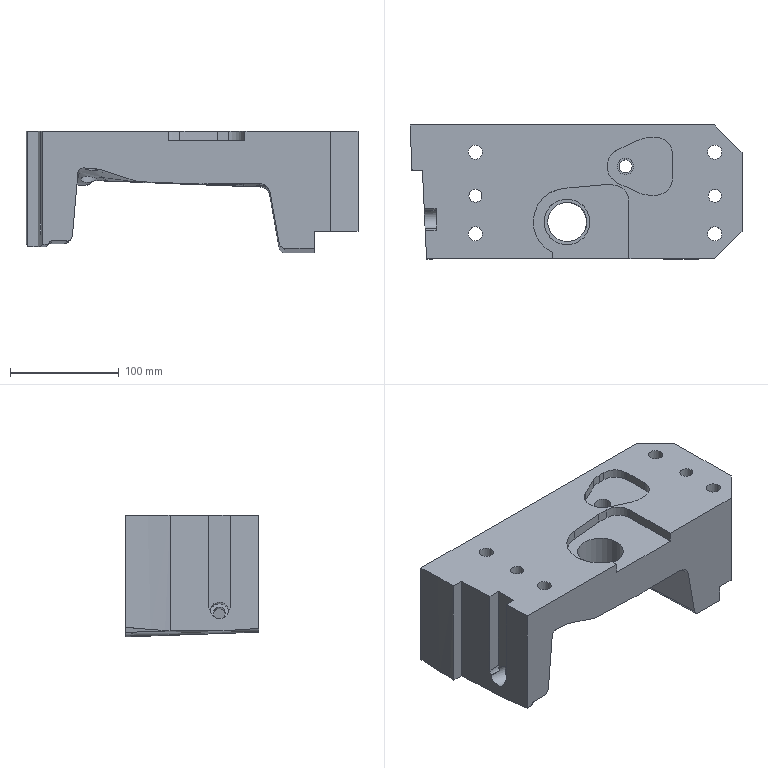Part | NX | features solid 2 | 1 solid | 144 faces | box 305.167 x 123.003 x 111.955 mm | volume 2142026 mm3 | spline 89 | plane 31 | cylinder 24 | commonest cylinder face diameters 20 x6 13 x4 12 x3 30 x3 50 x2 11 x1